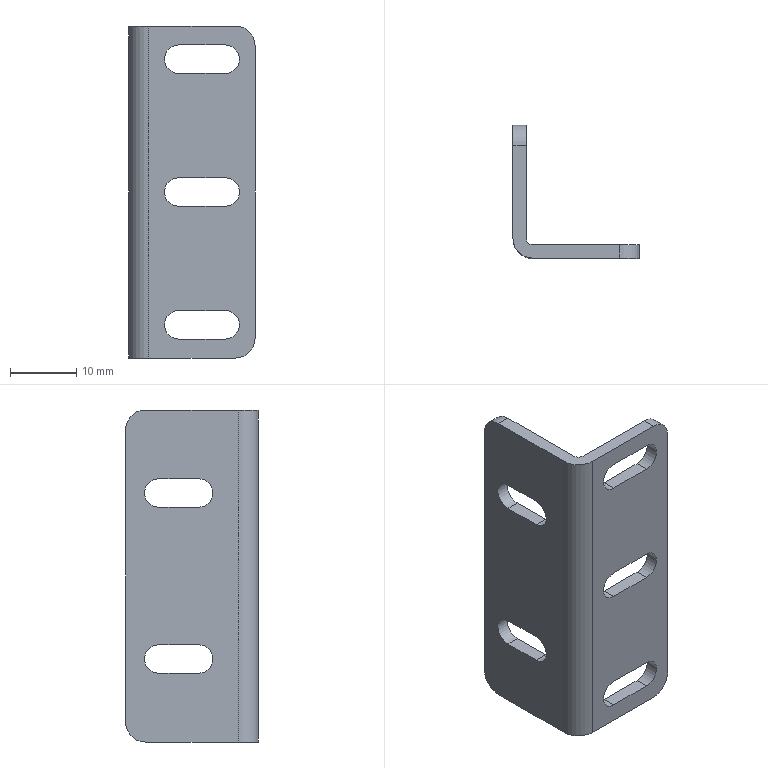Part | SolidWorks | features Fillet 3, ICE 2, ExtruThin 1 | 1 solid | 34 faces | box 19 x 20 x 50 mm | volume 3170 mm3 | plane 18 | cylinder 16 | commonest cylinder face diameters 4.3 x10 6 x5 2 x1
STEP:
#1=CARTESIAN_POINT('',(12.5,-2.,17.85));
#2=VERTEX_POINT('',#1);
#3=CARTESIAN_POINT('',(5.5,-2.,17.85));
#4=VERTEX_POINT('',#3);
#5=CARTESIAN_POINT('',(0.,-2.,17.85));
#6=DIRECTION('',(-1.,0.,0.));
#7=VECTOR('',#6,1000.);
#8=LINE('',#5,#7);
#9=EDGE_CURVE('',#2,#4,#8,.T.);
#10=ORIENTED_EDGE('',*,*,#9,.T.);
#11=CARTESIAN_POINT('',(5.5,-2.,22.15));
#12=VERTEX_POINT('',#11);
#13=CARTESIAN_POINT('',(5.5,-2.,20.));
#14=DIRECTION('',(0.,1.,0.));
#15=DIRECTION('',(0.,0.,1.));
#16=AXIS2_PLACEMENT_3D('',#13,#14,#15);
#17=CIRCLE('',#16,2.15);
#18=EDGE_CURVE('',#4,#12,#17,.T.);
#19=ORIENTED_EDGE('',*,*,#18,.T.);
#20=CARTESIAN_POINT('',(12.5,-2.,22.15));
#21=VERTEX_POINT('',#20);
#22=CARTESIAN_POINT('',(0.,-2.,22.15));
#23=DIRECTION('',(1.,0.,0.));
#24=VECTOR('',#23,1000.);
#25=LINE('',#22,#24);
#26=EDGE_CURVE('',#12,#21,#25,.T.);
#27=ORIENTED_EDGE('',*,*,#26,.T.);
#28=CARTESIAN_POINT('',(12.5,-2.,20.));
#29=DIRECTION('',(0.,1.,0.));
#30=DIRECTION('',(0.,0.,1.));
#31=AXIS2_PLACEMENT_3D('',#28,#29,#30);
#32=CIRCLE('',#31,2.15);
#33=EDGE_CURVE('',#21,#2,#32,.T.);
#34=ORIENTED_EDGE('',*,*,#33,.T.);
#35=EDGE_LOOP('',(#10,#19,#27,#34));
#36=FACE_BOUND('',#35,.T.);
#37=CARTESIAN_POINT('',(12.5,-2.,-2.15));
#38=VERTEX_POINT('',#37);
#39=CARTESIAN_POINT('',(5.5,-2.,-2.15));
#40=VERTEX_POINT('',#39);
#41=CARTESIAN_POINT('',(0.,-2.,-2.15));
#42=DIRECTION('',(-1.,0.,0.));
#43=VECTOR('',#42,1000.);
#44=LINE('',#41,#43);
#45=EDGE_CURVE('',#38,#40,#44,.T.);
#46=ORIENTED_EDGE('',*,*,#45,.T.);
#47=CARTESIAN_POINT('',(5.5,-2.,2.15));
#48=VERTEX_POINT('',#47);
#49=CARTESIAN_POINT('',(5.5,-2.,0.));
#50=DIRECTION('',(0.,1.,0.));
#51=DIRECTION('',(0.,0.,1.));
#52=AXIS2_PLACEMENT_3D('',#49,#50,#51);
#53=CIRCLE('',#52,2.15);
#54=EDGE_CURVE('',#40,#48,#53,.T.);
#55=ORIENTED_EDGE('',*,*,#54,.T.);
#56=CARTESIAN_POINT('',(12.5,-2.,2.15));
#57=VERTEX_POINT('',#56);
#58=CARTESIAN_POINT('',(0.,-2.,2.15));
#59=DIRECTION('',(1.,0.,0.));
#60=VECTOR('',#59,1000.);
#61=LINE('',#58,#60);
#62=EDGE_CURVE('',#48,#57,#61,.T.);
#63=ORIENTED_EDGE('',*,*,#62,.T.);
#64=CARTESIAN_POINT('',(12.5,-2.,0.));
#65=DIRECTION('',(0.,1.,0.));
#66=DIRECTION('',(0.,0.,1.));
#67=AXIS2_PLACEMENT_3D('',#64,#65,#66);
#68=CIRCLE('',#67,2.15);
#69=EDGE_CURVE('',#57,#38,#68,.T.);
#70=ORIENTED_EDGE('',*,*,#69,.T.);
#71=EDGE_LOOP('',(#46,#55,#63,#70));
#72=FACE_BOUND('',#71,.T.);
#73=CARTESIAN_POINT('',(12.5,-2.,-22.15));
#74=VERTEX_POINT('',#73);
#75=CARTESIAN_POINT('',(5.5,-2.,-22.15));
#76=VERTEX_POINT('',#75);
#77=CARTESIAN_POINT('',(0.,-2.,-22.15));
#78=DIRECTION('',(-1.,0.,0.));
#79=VECTOR('',#78,1000.);
#80=LINE('',#77,#79);
#81=EDGE_CURVE('',#74,#76,#80,.T.);
#82=ORIENTED_EDGE('',*,*,#81,.T.);
#83=CARTESIAN_POINT('',(5.5,-2.,-17.85));
#84=VERTEX_POINT('',#83);
#85=CARTESIAN_POINT('',(5.5,-2.,-20.));
#86=DIRECTION('',(0.,1.,0.));
#87=DIRECTION('',(0.,0.,1.));
#88=AXIS2_PLACEMENT_3D('',#85,#86,#87);
#89=CIRCLE('',#88,2.15);
#90=EDGE_CURVE('',#76,#84,#89,.T.);
#91=ORIENTED_EDGE('',*,*,#90,.T.);
#92=CARTESIAN_POINT('',(12.5,-2.,-17.85));
#93=VERTEX_POINT('',#92);
#94=CARTESIAN_POINT('',(0.,-2.,-17.85));
#95=DIRECTION('',(1.,0.,0.));
#96=VECTOR('',#95,1000.);
#97=LINE('',#94,#96);
#98=EDGE_CURVE('',#84,#93,#97,.T.);
#99=ORIENTED_EDGE('',*,*,#98,.T.);
#100=CARTESIAN_POINT('',(12.5,-2.,-20.));
#101=DIRECTION('',(0.,1.,0.));
#102=DIRECTION('',(0.,0.,1.));
#103=AXIS2_PLACEMENT_3D('',#100,#101,#102);
#104=CIRCLE('',#103,2.15);
#105=EDGE_CURVE('',#93,#74,#104,.T.);
#106=ORIENTED_EDGE('',*,*,#105,.T.);
#107=EDGE_LOOP('',(#82,#91,#99,#106));
#108=FACE_BOUND('',#107,.T.);
#109=CARTESIAN_POINT('',(1.,-2.,25.));
#110=VERTEX_POINT('',#109);
#111=CARTESIAN_POINT('',(14.,-2.,25.));
#112=VERTEX_POINT('',#111);
#113=CARTESIAN_POINT('',(0.,-2.,25.));
#114=DIRECTION('',(1.,0.,0.));
#115=VECTOR('',#114,1000.);
#116=LINE('',#113,#115);
#117=EDGE_CURVE('',#110,#112,#116,.T.);
#118=ORIENTED_EDGE('',*,*,#117,.F.);
#119=CARTESIAN_POINT('',(1.,-2.,-25.));
#120=VERTEX_POINT('',#119);
#121=CARTESIAN_POINT('',(1.,-2.,25.));
#122=DIRECTION('',(0.,0.,-1.));
#123=VECTOR('',#122,1000.);
#124=LINE('',#121,#123);
#125=EDGE_CURVE('',#110,#120,#124,.T.);
#126=ORIENTED_EDGE('',*,*,#125,.T.);
#127=CARTESIAN_POINT('',(14.,-2.,-25.));
#128=VERTEX_POINT('',#127);
#129=CARTESIAN_POINT('',(0.,-2.,-25.));
#130=DIRECTION('',(1.,0.,0.));
#131=VECTOR('',#130,1000.);
#132=LINE('',#129,#131);
#133=EDGE_CURVE('',#120,#128,#132,.T.);
#134=ORIENTED_EDGE('',*,*,#133,.T.);
#135=CARTESIAN_POINT('',(17.,-2.,-22.));
#136=VERTEX_POINT('',#135);
#137=CARTESIAN_POINT('',(14.,-2.,-22.));
#138=DIRECTION('',(0.,-1.,0.));
#139=DIRECTION('',(0.,0.,1.));
#140=AXIS2_PLACEMENT_3D('',#137,#138,#139);
#141=CIRCLE('',#140,3.);
#142=EDGE_CURVE('',#128,#136,#141,.T.);
#143=ORIENTED_EDGE('',*,*,#142,.T.);
#144=CARTESIAN_POINT('',(17.,-2.,22.));
#145=VERTEX_POINT('',#144);
#146=CARTESIAN_POINT('',(17.,-2.,25.));
#147=DIRECTION('',(0.,0.,-1.));
#148=VECTOR('',#147,1000.);
#149=LINE('',#146,#148);
#150=EDGE_CURVE('',#145,#136,#149,.T.);
#151=ORIENTED_EDGE('',*,*,#150,.F.);
#152=CARTESIAN_POINT('',(14.,-2.,22.));
#153=DIRECTION('',(0.,-1.,0.));
#154=DIRECTION('',(0.,0.,1.));
#155=AXIS2_PLACEMENT_3D('',#152,#153,#154);
#156=CIRCLE('',#155,3.);
#157=EDGE_CURVE('',#145,#112,#156,.T.);
#158=ORIENTED_EDGE('',*,*,#157,.T.);
#159=EDGE_LOOP('',(#118,#126,#134,#143,#151,#158));
#160=FACE_OUTER_BOUND('',#159,.T.);
#161=CARTESIAN_POINT('',(0.,-2.,25.));
#162=DIRECTION('',(0.,1.,0.));
#163=DIRECTION('',(0.,0.,1.));
#164=AXIS2_PLACEMENT_3D('',#161,#162,#163);
#165=PLANE('',#164);
#166=ADVANCED_FACE('',(#36,#72,#108,#160),#165,.F.);
#167=CARTESIAN_POINT('',(17.,0.,22.));
#168=VERTEX_POINT('',#167);
#169=CARTESIAN_POINT('',(17.,0.,-22.));
#170=VERTEX_POINT('',#169);
#171=CARTESIAN_POINT('',(17.,0.,25.));
#172=DIRECTION('',(0.,0.,-1.));
#173=VECTOR('',#172,1000.);
#174=LINE('',#171,#173);
#175=EDGE_CURVE('',#168,#170,#174,.T.);
#176=ORIENTED_EDGE('',*,*,#175,.F.);
#177=CARTESIAN_POINT('',(17.,-2.,22.));
#178=DIRECTION('',(0.,-1.,0.));
#179=VECTOR('',#178,1000.);
#180=LINE('',#177,#179);
#181=EDGE_CURVE('',#168,#145,#180,.T.);
#182=ORIENTED_EDGE('',*,*,#181,.T.);
#183=ORIENTED_EDGE('',*,*,#150,.T.);
#184=CARTESIAN_POINT('',(17.,0.,-22.));
#185=DIRECTION('',(0.,1.,0.));
#186=VECTOR('',#185,1000.);
#187=LINE('',#184,#186);
#188=EDGE_CURVE('',#136,#170,#187,.T.);
#189=ORIENTED_EDGE('',*,*,#188,.T.);
#190=EDGE_LOOP('',(#176,#182,#183,#189));
#191=FACE_OUTER_BOUND('',#190,.T.);
#192=CARTESIAN_POINT('',(17.,0.,25.));
#193=DIRECTION('',(1.,0.,0.));
#194=DIRECTION('',(0.,0.,-1.));
#195=AXIS2_PLACEMENT_3D('',#192,#193,#194);
#196=PLANE('',#195);
#197=ADVANCED_FACE('',(#191),#196,.T.);
#198=CARTESIAN_POINT('',(5.5,0.,17.85));
#199=VERTEX_POINT('',#198);
#200=CARTESIAN_POINT('',(5.5,0.,22.15));
#201=VERTEX_POINT('',#200);
#202=CARTESIAN_POINT('',(5.5,0.,20.));
#203=DIRECTION('',(0.,1.,0.));
#204=DIRECTION('',(0.,0.,-1.));
#205=AXIS2_PLACEMENT_3D('',#202,#203,#204);
#206=CIRCLE('',#205,2.15);
#207=EDGE_CURVE('',#199,#201,#206,.T.);
#208=ORIENTED_EDGE('',*,*,#207,.F.);
#209=CARTESIAN_POINT('',(12.5,0.,17.85));
#210=VERTEX_POINT('',#209);
#211=CARTESIAN_POINT('',(5.5,0.,17.85));
#212=DIRECTION('',(-1.,0.,0.));
#213=VECTOR('',#212,1000.);
#214=LINE('',#211,#213);
#215=EDGE_CURVE('',#210,#199,#214,.T.);
#216=ORIENTED_EDGE('',*,*,#215,.F.);
#217=CARTESIAN_POINT('',(12.5,0.,22.15));
#218=VERTEX_POINT('',#217);
#219=CARTESIAN_POINT('',(12.5,0.,20.));
#220=DIRECTION('',(0.,1.,0.));
#221=DIRECTION('',(0.,0.,-1.));
#222=AXIS2_PLACEMENT_3D('',#219,#220,#221);
#223=CIRCLE('',#222,2.15);
#224=EDGE_CURVE('',#218,#210,#223,.T.);
#225=ORIENTED_EDGE('',*,*,#224,.F.);
#226=CARTESIAN_POINT('',(5.5,0.,22.15));
#227=DIRECTION('',(1.,0.,0.));
#228=VECTOR('',#227,1000.);
#229=LINE('',#226,#228);
#230=EDGE_CURVE('',#201,#218,#229,.T.);
#231=ORIENTED_EDGE('',*,*,#230,.F.);
#232=EDGE_LOOP('',(#208,#216,#225,#231));
#233=FACE_BOUND('',#232,.T.);
#234=CARTESIAN_POINT('',(5.5,0.,-2.15));
#235=VERTEX_POINT('',#234);
#236=CARTESIAN_POINT('',(5.5,0.,2.15));
#237=VERTEX_POINT('',#236);
#238=CARTESIAN_POINT('',(5.5,0.,0.));
#239=DIRECTION('',(0.,1.,0.));
#240=DIRECTION('',(0.,0.,1.));
#241=AXIS2_PLACEMENT_3D('',#238,#239,#240);
#242=CIRCLE('',#241,2.15);
#243=EDGE_CURVE('',#235,#237,#242,.T.);
#244=ORIENTED_EDGE('',*,*,#243,.F.);
#245=CARTESIAN_POINT('',(12.5,0.,-2.15));
#246=VERTEX_POINT('',#245);
#247=CARTESIAN_POINT('',(5.5,0.,-2.15));
#248=DIRECTION('',(-1.,0.,0.));
#249=VECTOR('',#248,1000.);
#250=LINE('',#247,#249);
#251=EDGE_CURVE('',#246,#235,#250,.T.);
#252=ORIENTED_EDGE('',*,*,#251,.F.);
#253=CARTESIAN_POINT('',(12.5,0.,2.15));
#254=VERTEX_POINT('',#253);
#255=CARTESIAN_POINT('',(12.5,0.,0.));
#256=DIRECTION('',(0.,1.,0.));
#257=DIRECTION('',(0.,0.,1.));
#258=AXIS2_PLACEMENT_3D('',#255,#256,#257);
#259=CIRCLE('',#258,2.15);
#260=EDGE_CURVE('',#254,#246,#259,.T.);
#261=ORIENTED_EDGE('',*,*,#260,.F.);
#262=CARTESIAN_POINT('',(5.5,0.,2.15));
#263=DIRECTION('',(1.,0.,0.));
#264=VECTOR('',#263,1000.);
#265=LINE('',#262,#264);
#266=EDGE_CURVE('',#237,#254,#265,.T.);
#267=ORIENTED_EDGE('',*,*,#266,.F.);
#268=EDGE_LOOP('',(#244,#252,#261,#267));
#269=FACE_BOUND('',#268,.T.);
#270=CARTESIAN_POINT('',(5.5,0.,-22.15));
#271=VERTEX_POINT('',#270);
#272=CARTESIAN_POINT('',(5.5,0.,-17.85));
#273=VERTEX_POINT('',#272);
#274=CARTESIAN_POINT('',(5.5,0.,-20.));
#275=DIRECTION('',(0.,1.,0.));
#276=DIRECTION('',(0.,0.,1.));
#277=AXIS2_PLACEMENT_3D('',#274,#275,#276);
#278=CIRCLE('',#277,2.15);
#279=EDGE_CURVE('',#271,#273,#278,.T.);
#280=ORIENTED_EDGE('',*,*,#279,.F.);
#281=CARTESIAN_POINT('',(12.5,0.,-22.15));
#282=VERTEX_POINT('',#281);
#283=CARTESIAN_POINT('',(5.5,0.,-22.15));
#284=DIRECTION('',(-1.,0.,0.));
#285=VECTOR('',#284,1000.);
#286=LINE('',#283,#285);
#287=EDGE_CURVE('',#282,#271,#286,.T.);
#288=ORIENTED_EDGE('',*,*,#287,.F.);
#289=CARTESIAN_POINT('',(12.5,0.,-17.85));
#290=VERTEX_POINT('',#289);
#291=CARTESIAN_POINT('',(12.5,0.,-20.));
#292=DIRECTION('',(0.,1.,0.));
#293=DIRECTION('',(0.,0.,1.));
#294=AXIS2_PLACEMENT_3D('',#291,#292,#293);
#295=CIRCLE('',#294,2.15);
#296=EDGE_CURVE('',#290,#282,#295,.T.);
#297=ORIENTED_EDGE('',*,*,#296,.F.);
#298=CARTESIAN_POINT('',(5.5,0.,-17.85));
#299=DIRECTION('',(1.,0.,0.));
#300=VECTOR('',#299,1000.);
#301=LINE('',#298,#300);
#302=EDGE_CURVE('',#273,#290,#301,.T.);
#303=ORIENTED_EDGE('',*,*,#302,.F.);
#304=EDGE_LOOP('',(#280,#288,#297,#303));
#305=FACE_BOUND('',#304,.T.);
#306=CARTESIAN_POINT('',(1.,0.,-25.));
#307=VERTEX_POINT('',#306);
#308=CARTESIAN_POINT('',(14.,0.,-25.));
#309=VERTEX_POINT('',#308);
#310=CARTESIAN_POINT('',(0.,0.,-25.));
#311=DIRECTION('',(1.,0.,0.));
#312=VECTOR('',#311,1000.);
#313=LINE('',#310,#312);
#314=EDGE_CURVE('',#307,#309,#313,.T.);
#315=ORIENTED_EDGE('',*,*,#314,.F.);
#316=CARTESIAN_POINT('',(1.,0.,25.));
#317=VERTEX_POINT('',#316);
#318=CARTESIAN_POINT('',(1.,0.,25.));
#319=DIRECTION('',(0.,0.,1.));
#320=VECTOR('',#319,1000.);
#321=LINE('',#318,#320);
#322=EDGE_CURVE('',#307,#317,#321,.T.);
#323=ORIENTED_EDGE('',*,*,#322,.T.);
#324=CARTESIAN_POINT('',(14.,0.,25.));
#325=VERTEX_POINT('',#324);
#326=CARTESIAN_POINT('',(0.,0.,25.));
#327=DIRECTION('',(1.,0.,0.));
#328=VECTOR('',#327,1000.);
#329=LINE('',#326,#328);
#330=EDGE_CURVE('',#317,#325,#329,.T.);
#331=ORIENTED_EDGE('',*,*,#330,.T.);
#332=CARTESIAN_POINT('',(14.,0.,22.));
#333=DIRECTION('',(0.,1.,0.));
#334=DIRECTION('',(0.,0.,1.));
#335=AXIS2_PLACEMENT_3D('',#332,#333,#334);
#336=CIRCLE('',#335,3.);
#337=EDGE_CURVE('',#325,#168,#336,.T.);
#338=ORIENTED_EDGE('',*,*,#337,.T.);
#339=ORIENTED_EDGE('',*,*,#175,.T.);
#340=CARTESIAN_POINT('',(14.,0.,-22.));
#341=DIRECTION('',(0.,1.,0.));
#342=DIRECTION('',(0.,0.,1.));
#343=AXIS2_PLACEMENT_3D('',#340,#341,#342);
#344=CIRCLE('',#343,3.);
#345=EDGE_CURVE('',#170,#309,#344,.T.);
#346=ORIENTED_EDGE('',*,*,#345,.T.);
#347=EDGE_LOOP('',(#315,#323,#331,#338,#339,#346));
#348=FACE_OUTER_BOUND('',#347,.T.);
#349=CARTESIAN_POINT('',(0.,0.,25.));
#350=DIRECTION('',(0.,1.,0.));
#351=DIRECTION('',(0.,0.,1.));
#352=AXIS2_PLACEMENT_3D('',#349,#350,#351);
#353=PLANE('',#352);
#354=ADVANCED_FACE('',(#233,#269,#305,#348),#353,.T.);
#355=CARTESIAN_POINT('',(0.,13.,-14.65));
#356=VERTEX_POINT('',#355);
#357=CARTESIAN_POINT('',(0.,13.,-10.35));
#358=VERTEX_POINT('',#357);
#359=CARTESIAN_POINT('',(0.,13.,-12.5));
#360=DIRECTION('',(1.,0.,0.));
#361=DIRECTION('',(0.,0.,1.));
#362=AXIS2_PLACEMENT_3D('',#359,#360,#361);
#363=CIRCLE('',#362,2.15);
#364=EDGE_CURVE('',#356,#358,#363,.T.);
#365=ORIENTED_EDGE('',*,*,#364,.F.);
#366=CARTESIAN_POINT('',(0.,7.,-14.65));
#367=VERTEX_POINT('',#366);
#368=CARTESIAN_POINT('',(0.,13.,-14.65));
#369=DIRECTION('',(0.,1.,0.));
#370=VECTOR('',#369,1000.);
#371=LINE('',#368,#370);
#372=EDGE_CURVE('',#367,#356,#371,.T.);
#373=ORIENTED_EDGE('',*,*,#372,.F.);
#374=CARTESIAN_POINT('',(0.,7.,-10.35));
#375=VERTEX_POINT('',#374);
#376=CARTESIAN_POINT('',(0.,7.,-12.5));
#377=DIRECTION('',(1.,0.,0.));
#378=DIRECTION('',(0.,0.,1.));
#379=AXIS2_PLACEMENT_3D('',#376,#377,#378);
#380=CIRCLE('',#379,2.15);
#381=EDGE_CURVE('',#375,#367,#380,.T.);
#382=ORIENTED_EDGE('',*,*,#381,.F.);
#383=CARTESIAN_POINT('',(0.,13.,-10.35));
#384=DIRECTION('',(0.,-1.,0.));
#385=VECTOR('',#384,1000.);
#386=LINE('',#383,#385);
#387=EDGE_CURVE('',#358,#375,#386,.T.);
#388=ORIENTED_EDGE('',*,*,#387,.F.);
#389=EDGE_LOOP('',(#365,#373,#382,#388));
#390=FACE_BOUND('',#389,.T.);
#391=CARTESIAN_POINT('',(0.,13.,10.35));
#392=VERTEX_POINT('',#391);
#393=CARTESIAN_POINT('',(0.,13.,14.65));
#394=VERTEX_POINT('',#393);
#395=CARTESIAN_POINT('',(0.,13.,12.5));
#396=DIRECTION('',(1.,0.,0.));
#397=DIRECTION('',(0.,0.,-1.));
#398=AXIS2_PLACEMENT_3D('',#395,#396,#397);
#399=CIRCLE('',#398,2.15);
#400=EDGE_CURVE('',#392,#394,#399,.T.);
#401=ORIENTED_EDGE('',*,*,#400,.F.);
#402=CARTESIAN_POINT('',(0.,7.,10.35));
#403=VERTEX_POINT('',#402);
#404=CARTESIAN_POINT('',(0.,13.,10.35));
#405=DIRECTION('',(0.,1.,0.));
#406=VECTOR('',#405,1000.);
#407=LINE('',#404,#406);
#408=EDGE_CURVE('',#403,#392,#407,.T.);
#409=ORIENTED_EDGE('',*,*,#408,.F.);
#410=CARTESIAN_POINT('',(0.,7.,14.65));
#411=VERTEX_POINT('',#410);
#412=CARTESIAN_POINT('',(0.,7.,12.5));
#413=DIRECTION('',(1.,0.,0.));
#414=DIRECTION('',(0.,0.,-1.));
#415=AXIS2_PLACEMENT_3D('',#412,#413,#414);
#416=CIRCLE('',#415,2.15);
#417=EDGE_CURVE('',#411,#403,#416,.T.);
#418=ORIENTED_EDGE('',*,*,#417,.F.);
#419=CARTESIAN_POINT('',(0.,13.,14.65));
#420=DIRECTION('',(0.,-1.,0.));
#421=VECTOR('',#420,1000.);
#422=LINE('',#419,#421);
#423=EDGE_CURVE('',#394,#411,#422,.T.);
#424=ORIENTED_EDGE('',*,*,#423,.F.);
#425=EDGE_LOOP('',(#401,#409,#418,#424));
#426=FACE_BOUND('',#425,.T.);
#427=CARTESIAN_POINT('',(0.,15.,25.));
#428=VERTEX_POINT('',#427);
#429=CARTESIAN_POINT('',(0.,1.,25.));
#430=VERTEX_POINT('',#429);
#431=CARTESIAN_POINT('',(0.,0.,25.));
#432=DIRECTION('',(0.,-1.,0.));
#433=VECTOR('',#432,1000.);
#434=LINE('',#431,#433);
#435=EDGE_CURVE('',#428,#430,#434,.T.);
#436=ORIENTED_EDGE('',*,*,#435,.T.);
#437=CARTESIAN_POINT('',(0.,1.,-25.));
#438=VERTEX_POINT('',#437);
#439=CARTESIAN_POINT('',(0.,1.,-25.));
#440=DIRECTION('',(0.,0.,-1.));
#441=VECTOR('',#440,1000.);
#442=LINE('',#439,#441);
#443=EDGE_CURVE('',#430,#438,#442,.T.);
#444=ORIENTED_EDGE('',*,*,#443,.T.);
#445=CARTESIAN_POINT('',(0.,15.,-25.));
#446=VERTEX_POINT('',#445);
#447=CARTESIAN_POINT('',(0.,0.,-25.));
#448=DIRECTION('',(0.,-1.,0.));
#449=VECTOR('',#448,1000.);
#450=LINE('',#447,#449);
#451=EDGE_CURVE('',#446,#438,#450,.T.);
#452=ORIENTED_EDGE('',*,*,#451,.F.);
#453=CARTESIAN_POINT('',(0.,18.,-22.));
#454=VERTEX_POINT('',#453);
#455=CARTESIAN_POINT('',(0.,15.,-22.));
#456=DIRECTION('',(1.,0.,0.));
#457=DIRECTION('',(0.,0.,-1.));
#458=AXIS2_PLACEMENT_3D('',#455,#456,#457);
#459=CIRCLE('',#458,3.);
#460=EDGE_CURVE('',#446,#454,#459,.T.);
#461=ORIENTED_EDGE('',*,*,#460,.T.);
#462=CARTESIAN_POINT('',(0.,18.,22.));
#463=VERTEX_POINT('',#462);
#464=CARTESIAN_POINT('',(0.,18.,25.));
#465=DIRECTION('',(0.,0.,-1.));
#466=VECTOR('',#465,1000.);
#467=LINE('',#464,#466);
#468=EDGE_CURVE('',#463,#454,#467,.T.);
#469=ORIENTED_EDGE('',*,*,#468,.F.);
#470=CARTESIAN_POINT('',(0.,15.,22.));
#471=DIRECTION('',(1.,0.,0.));
#472=DIRECTION('',(0.,0.,-1.));
#473=AXIS2_PLACEMENT_3D('',#470,#471,#472);
#474=CIRCLE('',#473,3.);
#475=EDGE_CURVE('',#463,#428,#474,.T.);
#476=ORIENTED_EDGE('',*,*,#475,.T.);
#477=EDGE_LOOP('',(#436,#444,#452,#461,#469,#476));
#478=FACE_OUTER_BOUND('',#477,.T.);
#479=CARTESIAN_POINT('',(0.,0.,25.));
#480=DIRECTION('',(1.,0.,0.));
#481=DIRECTION('',(0.,0.,-1.));
#482=AXIS2_PLACEMENT_3D('',#479,#480,#481);
#483=PLANE('',#482);
#484=ADVANCED_FACE('',(#390,#426,#478),#483,.T.);
#485=CARTESIAN_POINT('',(-2.,18.,22.));
#486=VERTEX_POINT('',#485);
#487=CARTESIAN_POINT('',(-2.,18.,-22.));
#488=VERTEX_POINT('',#487);
#489=CARTESIAN_POINT('',(-2.,18.,25.));
#490=DIRECTION('',(0.,0.,-1.));
#491=VECTOR('',#490,1000.);
#492=LINE('',#489,#491);
#493=EDGE_CURVE('',#486,#488,#492,.T.);
#494=ORIENTED_EDGE('',*,*,#493,.F.);
#495=CARTESIAN_POINT('',(0.,18.,22.));
#496=DIRECTION('',(1.,0.,0.));
#497=VECTOR('',#496,1000.);
#498=LINE('',#495,#497);
#499=EDGE_CURVE('',#486,#463,#498,.T.);
#500=ORIENTED_EDGE('',*,*,#499,.T.);
#501=ORIENTED_EDGE('',*,*,#468,.T.);
#502=CARTESIAN_POINT('',(-2.,18.,-22.));
#503=DIRECTION('',(-1.,0.,0.));
#504=VECTOR('',#503,1000.);
#505=LINE('',#502,#504);
#506=EDGE_CURVE('',#454,#488,#505,.T.);
#507=ORIENTED_EDGE('',*,*,#506,.T.);
#508=EDGE_LOOP('',(#494,#500,#501,#507));
#509=FACE_OUTER_BOUND('',#508,.T.);
#510=CARTESIAN_POINT('',(-2.,18.,25.));
#511=DIRECTION('',(0.,1.,0.));
#512=DIRECTION('',(0.,0.,1.));
#513=AXIS2_PLACEMENT_3D('',#510,#511,#512);
#514=PLANE('',#513);
#515=ADVANCED_FACE('',(#509),#514,.T.);
#516=CARTESIAN_POINT('',(-2.,7.,-14.65));
#517=VERTEX_POINT('',#516);
#518=CARTESIAN_POINT('',(-2.,13.,-14.65));
#519=VERTEX_POINT('',#518);
#520=CARTESIAN_POINT('',(-2.,0.,-14.65));
#521=DIRECTION('',(0.,1.,0.));
#522=VECTOR('',#521,1000.);
#523=LINE('',#520,#522);
#524=EDGE_CURVE('',#517,#519,#523,.T.);
#525=ORIENTED_EDGE('',*,*,#524,.T.);
#526=CARTESIAN_POINT('',(-2.,13.,-10.35));
#527=VERTEX_POINT('',#526);
#528=CARTESIAN_POINT('',(-2.,13.,-12.5));
#529=DIRECTION('',(1.,0.,0.));
#530=DIRECTION('',(0.,0.,-1.));
#531=AXIS2_PLACEMENT_3D('',#528,#529,#530);
#532=CIRCLE('',#531,2.15);
#533=EDGE_CURVE('',#519,#527,#532,.T.);
#534=ORIENTED_EDGE('',*,*,#533,.T.);
#535=CARTESIAN_POINT('',(-2.,7.,-10.35));
#536=VERTEX_POINT('',#535);
#537=CARTESIAN_POINT('',(-2.,0.,-10.35));
#538=DIRECTION('',(0.,-1.,0.));
#539=VECTOR('',#538,1000.);
#540=LINE('',#537,#539);
#541=EDGE_CURVE('',#527,#536,#540,.T.);
#542=ORIENTED_EDGE('',*,*,#541,.T.);
#543=CARTESIAN_POINT('',(-2.,7.,-12.5));
#544=DIRECTION('',(1.,0.,0.));
#545=DIRECTION('',(0.,0.,-1.));
#546=AXIS2_PLACEMENT_3D('',#543,#544,#545);
#547=CIRCLE('',#546,2.15);
#548=EDGE_CURVE('',#536,#517,#547,.T.);
#549=ORIENTED_EDGE('',*,*,#548,.T.);
#550=EDGE_LOOP('',(#525,#534,#542,#549));
#551=FACE_BOUND('',#550,.T.);
#552=CARTESIAN_POINT('',(-2.,7.,10.35));
#553=VERTEX_POINT('',#552);
#554=CARTESIAN_POINT('',(-2.,13.,10.35));
#555=VERTEX_POINT('',#554);
#556=CARTESIAN_POINT('',(-2.,0.,10.35));
#557=DIRECTION('',(0.,1.,0.));
#558=VECTOR('',#557,1000.);
#559=LINE('',#556,#558);
#560=EDGE_CURVE('',#553,#555,#559,.T.);
#561=ORIENTED_EDGE('',*,*,#560,.T.);
#562=CARTESIAN_POINT('',(-2.,13.,14.65));
#563=VERTEX_POINT('',#562);
#564=CARTESIAN_POINT('',(-2.,13.,12.5));
#565=DIRECTION('',(1.,0.,0.));
#566=DIRECTION('',(0.,0.,-1.));
#567=AXIS2_PLACEMENT_3D('',#564,#565,#566);
#568=CIRCLE('',#567,2.15);
#569=EDGE_CURVE('',#555,#563,#568,.T.);
#570=ORIENTED_EDGE('',*,*,#569,.T.);
#571=CARTESIAN_POINT('',(-2.,7.,14.65));
#572=VERTEX_POINT('',#571);
#573=CARTESIAN_POINT('',(-2.,0.,14.65));
#574=DIRECTION('',(0.,-1.,0.));
#575=VECTOR('',#574,1000.);
#576=LINE('',#573,#575);
#577=EDGE_CURVE('',#563,#572,#576,.T.);
#578=ORIENTED_EDGE('',*,*,#577,.T.);
#579=CARTESIAN_POINT('',(-2.,7.,12.5));
#580=DIRECTION('',(1.,0.,0.));
#581=DIRECTION('',(0.,0.,-1.));
#582=AXIS2_PLACEMENT_3D('',#579,#580,#581);
#583=CIRCLE('',#582,2.15);
#584=EDGE_CURVE('',#572,#553,#583,.T.);
#585=ORIENTED_EDGE('',*,*,#584,.T.);
#586=EDGE_LOOP('',(#561,#570,#578,#585));
#587=FACE_BOUND('',#586,.T.);
#588=CARTESIAN_POINT('',(-2.,15.,-25.));
#589=VERTEX_POINT('',#588);
#590=CARTESIAN_POINT('',(-2.,1.,-25.));
#591=VERTEX_POINT('',#590);
#592=CARTESIAN_POINT('',(-2.,0.,-25.));
#593=DIRECTION('',(0.,-1.,0.));
#594=VECTOR('',#593,1000.);
#595=LINE('',#592,#594);
#596=EDGE_CURVE('',#589,#591,#595,.T.);
#597=ORIENTED_EDGE('',*,*,#596,.T.);
#598=CARTESIAN_POINT('',(-2.,1.,25.));
#599=VERTEX_POINT('',#598);
#600=CARTESIAN_POINT('',(-2.,1.,25.));
#601=DIRECTION('',(0.,0.,1.));
#602=VECTOR('',#601,1000.);
#603=LINE('',#600,#602);
#604=EDGE_CURVE('',#591,#599,#603,.T.);
#605=ORIENTED_EDGE('',*,*,#604,.T.);
#606=CARTESIAN_POINT('',(-2.,15.,25.));
#607=VERTEX_POINT('',#606);
#608=CARTESIAN_POINT('',(-2.,0.,25.));
#609=DIRECTION('',(0.,-1.,0.));
#610=VECTOR('',#609,1000.);
#611=LINE('',#608,#610);
#612=EDGE_CURVE('',#607,#599,#611,.T.);
#613=ORIENTED_EDGE('',*,*,#612,.F.);
#614=CARTESIAN_POINT('',(-2.,15.,22.));
#615=DIRECTION('',(-1.,0.,0.));
#616=DIRECTION('',(0.,0.,-1.));
#617=AXIS2_PLACEMENT_3D('',#614,#615,#616);
#618=CIRCLE('',#617,3.);
#619=EDGE_CURVE('',#607,#486,#618,.T.);
#620=ORIENTED_EDGE('',*,*,#619,.T.);
#621=ORIENTED_EDGE('',*,*,#493,.T.);
#622=CARTESIAN_POINT('',(-2.,15.,-22.));
#623=DIRECTION('',(-1.,0.,0.));
#624=DIRECTION('',(0.,0.,-1.));
#625=AXIS2_PLACEMENT_3D('',#622,#623,#624);
#626=CIRCLE('',#625,3.);
#627=EDGE_CURVE('',#488,#589,#626,.T.);
#628=ORIENTED_EDGE('',*,*,#627,.T.);
#629=EDGE_LOOP('',(#597,#605,#613,#620,#621,#628));
#630=FACE_OUTER_BOUND('',#629,.T.);
#631=CARTESIAN_POINT('',(-2.,0.,25.));
#632=DIRECTION('',(1.,0.,0.));
#633=DIRECTION('',(0.,0.,-1.));
#634=AXIS2_PLACEMENT_3D('',#631,#632,#633);
#635=PLANE('',#634);
#636=ADVANCED_FACE('',(#551,#587,#630),#635,.F.);
#637=ORIENTED_EDGE('',*,*,#612,.T.);
#638=CARTESIAN_POINT('',(1.,1.,25.));
#639=DIRECTION('',(0.,0.,1.));
#640=DIRECTION('',(-1.,0.,0.));
#641=AXIS2_PLACEMENT_3D('',#638,#639,#640);
#642=CIRCLE('',#641,3.);
#643=EDGE_CURVE('',#599,#110,#642,.T.);
#644=ORIENTED_EDGE('',*,*,#643,.T.);
#645=ORIENTED_EDGE('',*,*,#117,.T.);
#646=CARTESIAN_POINT('',(14.,0.,25.));
#647=DIRECTION('',(0.,1.,0.));
#648=VECTOR('',#647,1000.);
#649=LINE('',#646,#648);
#650=EDGE_CURVE('',#112,#325,#649,.T.);
#651=ORIENTED_EDGE('',*,*,#650,.T.);
#652=ORIENTED_EDGE('',*,*,#330,.F.);
#653=CARTESIAN_POINT('',(1.,1.,25.));
#654=DIRECTION('',(0.,0.,-1.));
#655=DIRECTION('',(-1.,0.,0.));
#656=AXIS2_PLACEMENT_3D('',#653,#654,#655);
#657=CIRCLE('',#656,1.);
#658=EDGE_CURVE('',#317,#430,#657,.T.);
#659=ORIENTED_EDGE('',*,*,#658,.T.);
#660=ORIENTED_EDGE('',*,*,#435,.F.);
#661=CARTESIAN_POINT('',(-2.,15.,25.));
#662=DIRECTION('',(-1.,0.,0.));
#663=VECTOR('',#662,1000.);
#664=LINE('',#661,#663);
#665=EDGE_CURVE('',#428,#607,#664,.T.);
#666=ORIENTED_EDGE('',*,*,#665,.T.);
#667=EDGE_LOOP('',(#637,#644,#645,#651,#652,#659,#660,#666));
#668=FACE_OUTER_BOUND('',#667,.T.);
#669=CARTESIAN_POINT('',(0.,0.,25.));
#670=DIRECTION('',(0.,0.,-1.));
#671=DIRECTION('',(-1.,0.,0.));
#672=AXIS2_PLACEMENT_3D('',#669,#670,#671);
#673=PLANE('',#672);
#674=ADVANCED_FACE('',(#668),#673,.F.);
#675=ORIENTED_EDGE('',*,*,#133,.F.);
#676=CARTESIAN_POINT('',(1.,1.,-25.));
#677=DIRECTION('',(0.,0.,-1.));
#678=DIRECTION('',(-1.,0.,0.));
#679=AXIS2_PLACEMENT_3D('',#676,#677,#678);
#680=CIRCLE('',#679,3.);
#681=EDGE_CURVE('',#120,#591,#680,.T.);
#682=ORIENTED_EDGE('',*,*,#681,.T.);
#683=ORIENTED_EDGE('',*,*,#596,.F.);
#684=CARTESIAN_POINT('',(0.,15.,-25.));
#685=DIRECTION('',(1.,0.,0.));
#686=VECTOR('',#685,1000.);
#687=LINE('',#684,#686);
#688=EDGE_CURVE('',#589,#446,#687,.T.);
#689=ORIENTED_EDGE('',*,*,#688,.T.);
#690=ORIENTED_EDGE('',*,*,#451,.T.);
#691=CARTESIAN_POINT('',(1.,1.,-25.));
#692=DIRECTION('',(0.,0.,1.));
#693=DIRECTION('',(-1.,0.,0.));
#694=AXIS2_PLACEMENT_3D('',#691,#692,#693);
#695=CIRCLE('',#694,1.);
#696=EDGE_CURVE('',#438,#307,#695,.T.);
#697=ORIENTED_EDGE('',*,*,#696,.T.);
#698=ORIENTED_EDGE('',*,*,#314,.T.);
#699=CARTESIAN_POINT('',(14.,0.,-25.));
#700=DIRECTION('',(0.,-1.,0.));
#701=VECTOR('',#700,1000.);
#702=LINE('',#699,#701);
#703=EDGE_CURVE('',#309,#128,#702,.T.);
#704=ORIENTED_EDGE('',*,*,#703,.T.);
#705=EDGE_LOOP('',(#675,#682,#683,#689,#690,#697,#698,#704));
#706=FACE_OUTER_BOUND('',#705,.T.);
#707=CARTESIAN_POINT('',(0.,0.,-25.));
#708=DIRECTION('',(0.,0.,-1.));
#709=DIRECTION('',(-1.,0.,0.));
#710=AXIS2_PLACEMENT_3D('',#707,#708,#709);
#711=PLANE('',#710);
#712=ADVANCED_FACE('',(#706),#711,.T.);
#713=CARTESIAN_POINT('',(5.5,-10.,-22.15));
#714=DIRECTION('',(0.,1.,0.));
#715=VECTOR('',#714,1000.);
#716=LINE('',#713,#715);
#717=EDGE_CURVE('',#76,#271,#716,.T.);
#718=ORIENTED_EDGE('',*,*,#717,.T.);
#719=ORIENTED_EDGE('',*,*,#279,.T.);
#720=CARTESIAN_POINT('',(5.5,-10.,-17.85));
#721=DIRECTION('',(0.,1.,0.));
#722=VECTOR('',#721,1000.);
#723=LINE('',#720,#722);
#724=EDGE_CURVE('',#84,#273,#723,.T.);
#725=ORIENTED_EDGE('',*,*,#724,.F.);
#726=ORIENTED_EDGE('',*,*,#90,.F.);
#727=EDGE_LOOP('',(#718,#719,#725,#726));
#728=FACE_OUTER_BOUND('',#727,.T.);
#729=CARTESIAN_POINT('',(5.5,-10.,-20.));
#730=DIRECTION('',(0.,1.,0.));
#731=DIRECTION('',(0.,0.,1.));
#732=AXIS2_PLACEMENT_3D('',#729,#730,#731);
#733=CYLINDRICAL_SURFACE('',#732,2.15);
#734=ADVANCED_FACE('',(#728),#733,.F.);
#735=CARTESIAN_POINT('',(12.5,-10.,-22.15));
#736=DIRECTION('',(0.,1.,0.));
#737=VECTOR('',#736,1000.);
#738=LINE('',#735,#737);
#739=EDGE_CURVE('',#74,#282,#738,.T.);
#740=ORIENTED_EDGE('',*,*,#739,.T.);
#741=ORIENTED_EDGE('',*,*,#287,.T.);
#742=ORIENTED_EDGE('',*,*,#717,.F.);
#743=ORIENTED_EDGE('',*,*,#81,.F.);
#744=EDGE_LOOP('',(#740,#741,#742,#743));
#745=FACE_OUTER_BOUND('',#744,.T.);
#746=CARTESIAN_POINT('',(5.5,-10.,-22.15));
#747=DIRECTION('',(0.,0.,-1.));
#748=DIRECTION('',(-1.,0.,0.));
#749=AXIS2_PLACEMENT_3D('',#746,#747,#748);
#750=PLANE('',#749);
#751=ADVANCED_FACE('',(#745),#750,.F.);
#752=CARTESIAN_POINT('',(12.5,-10.,-17.85));
#753=DIRECTION('',(0.,1.,0.));
#754=VECTOR('',#753,1000.);
#755=LINE('',#752,#754);
#756=EDGE_CURVE('',#93,#290,#755,.T.);
#757=ORIENTED_EDGE('',*,*,#756,.T.);
#758=ORIENTED_EDGE('',*,*,#296,.T.);
#759=ORIENTED_EDGE('',*,*,#739,.F.);
#760=ORIENTED_EDGE('',*,*,#105,.F.);
#761=EDGE_LOOP('',(#757,#758,#759,#760));
#762=FACE_OUTER_BOUND('',#761,.T.);
#763=CARTESIAN_POINT('',(12.5,-10.,-20.));
#764=DIRECTION('',(0.,1.,0.));
#765=DIRECTION('',(0.,0.,1.));
#766=AXIS2_PLACEMENT_3D('',#763,#764,#765);
#767=CYLINDRICAL_SURFACE('',#766,2.15);
#768=ADVANCED_FACE('',(#762),#767,.F.);
#769=ORIENTED_EDGE('',*,*,#724,.T.);
#770=ORIENTED_EDGE('',*,*,#302,.T.);
#771=ORIENTED_EDGE('',*,*,#756,.F.);
#772=ORIENTED_EDGE('',*,*,#98,.F.);
#773=EDGE_LOOP('',(#769,#770,#771,#772));
#774=FACE_OUTER_BOUND('',#773,.T.);
#775=CARTESIAN_POINT('',(5.5,-10.,-17.85));
#776=DIRECTION('',(0.,0.,1.));
#777=DIRECTION('',(1.,0.,0.));
#778=AXIS2_PLACEMENT_3D('',#775,#776,#777);
#779=PLANE('',#778);
#780=ADVANCED_FACE('',(#774),#779,.F.);
#781=CARTESIAN_POINT('',(5.5,-10.,-2.15));
#782=DIRECTION('',(0.,1.,0.));
#783=VECTOR('',#782,1000.);
#784=LINE('',#781,#783);
#785=EDGE_CURVE('',#40,#235,#784,.T.);
#786=ORIENTED_EDGE('',*,*,#785,.T.);
#787=ORIENTED_EDGE('',*,*,#243,.T.);
#788=CARTESIAN_POINT('',(5.5,-10.,2.15));
#789=DIRECTION('',(0.,1.,0.));
#790=VECTOR('',#789,1000.);
#791=LINE('',#788,#790);
#792=EDGE_CURVE('',#48,#237,#791,.T.);
#793=ORIENTED_EDGE('',*,*,#792,.F.);
#794=ORIENTED_EDGE('',*,*,#54,.F.);
#795=EDGE_LOOP('',(#786,#787,#793,#794));
#796=FACE_OUTER_BOUND('',#795,.T.);
#797=CARTESIAN_POINT('',(5.5,-10.,0.));
#798=DIRECTION('',(0.,1.,0.));
#799=DIRECTION('',(0.,0.,1.));
#800=AXIS2_PLACEMENT_3D('',#797,#798,#799);
#801=CYLINDRICAL_SURFACE('',#800,2.15);
#802=ADVANCED_FACE('',(#796),#801,.F.);
#803=CARTESIAN_POINT('',(12.5,-10.,-2.15));
#804=DIRECTION('',(0.,1.,0.));
#805=VECTOR('',#804,1000.);
#806=LINE('',#803,#805);
#807=EDGE_CURVE('',#38,#246,#806,.T.);
#808=ORIENTED_EDGE('',*,*,#807,.T.);
#809=ORIENTED_EDGE('',*,*,#251,.T.);
#810=ORIENTED_EDGE('',*,*,#785,.F.);
#811=ORIENTED_EDGE('',*,*,#45,.F.);
#812=EDGE_LOOP('',(#808,#809,#810,#811));
#813=FACE_OUTER_BOUND('',#812,.T.);
#814=CARTESIAN_POINT('',(5.5,-10.,-2.15));
#815=DIRECTION('',(0.,0.,-1.));
#816=DIRECTION('',(-1.,0.,0.));
#817=AXIS2_PLACEMENT_3D('',#814,#815,#816);
#818=PLANE('',#817);
#819=ADVANCED_FACE('',(#813),#818,.F.);
#820=CARTESIAN_POINT('',(12.5,-10.,2.15));
#821=DIRECTION('',(0.,1.,0.));
#822=VECTOR('',#821,1000.);
#823=LINE('',#820,#822);
#824=EDGE_CURVE('',#57,#254,#823,.T.);
#825=ORIENTED_EDGE('',*,*,#824,.T.);
#826=ORIENTED_EDGE('',*,*,#260,.T.);
#827=ORIENTED_EDGE('',*,*,#807,.F.);
#828=ORIENTED_EDGE('',*,*,#69,.F.);
#829=EDGE_LOOP('',(#825,#826,#827,#828));
#830=FACE_OUTER_BOUND('',#829,.T.);
#831=CARTESIAN_POINT('',(12.5,-10.,0.));
#832=DIRECTION('',(0.,1.,0.));
#833=DIRECTION('',(0.,0.,1.));
#834=AXIS2_PLACEMENT_3D('',#831,#832,#833);
#835=CYLINDRICAL_SURFACE('',#834,2.15);
#836=ADVANCED_FACE('',(#830),#835,.F.);
#837=ORIENTED_EDGE('',*,*,#792,.T.);
#838=ORIENTED_EDGE('',*,*,#266,.T.);
#839=ORIENTED_EDGE('',*,*,#824,.F.);
#840=ORIENTED_EDGE('',*,*,#62,.F.);
#841=EDGE_LOOP('',(#837,#838,#839,#840));
#842=FACE_OUTER_BOUND('',#841,.T.);
#843=CARTESIAN_POINT('',(5.5,-10.,2.15));
#844=DIRECTION('',(0.,0.,1.));
#845=DIRECTION('',(1.,0.,0.));
#846=AXIS2_PLACEMENT_3D('',#843,#844,#845);
#847=PLANE('',#846);
#848=ADVANCED_FACE('',(#842),#847,.F.);
#849=CARTESIAN_POINT('',(5.5,-10.,17.85));
#850=DIRECTION('',(0.,1.,0.));
#851=VECTOR('',#850,1000.);
#852=LINE('',#849,#851);
#853=EDGE_CURVE('',#4,#199,#852,.T.);
#854=ORIENTED_EDGE('',*,*,#853,.T.);
#855=ORIENTED_EDGE('',*,*,#207,.T.);
#856=CARTESIAN_POINT('',(5.5,-10.,22.15));
#857=DIRECTION('',(0.,1.,0.));
#858=VECTOR('',#857,1000.);
#859=LINE('',#856,#858);
#860=EDGE_CURVE('',#12,#201,#859,.T.);
#861=ORIENTED_EDGE('',*,*,#860,.F.);
#862=ORIENTED_EDGE('',*,*,#18,.F.);
#863=EDGE_LOOP('',(#854,#855,#861,#862));
#864=FACE_OUTER_BOUND('',#863,.T.);
#865=CARTESIAN_POINT('',(5.5,-10.,20.));
#866=DIRECTION('',(0.,1.,0.));
#867=DIRECTION('',(0.,0.,1.));
#868=AXIS2_PLACEMENT_3D('',#865,#866,#867);
#869=CYLINDRICAL_SURFACE('',#868,2.15);
#870=ADVANCED_FACE('',(#864),#869,.F.);
#871=CARTESIAN_POINT('',(12.5,-10.,17.85));
#872=DIRECTION('',(0.,1.,0.));
#873=VECTOR('',#872,1000.);
#874=LINE('',#871,#873);
#875=EDGE_CURVE('',#2,#210,#874,.T.);
#876=ORIENTED_EDGE('',*,*,#875,.T.);
#877=ORIENTED_EDGE('',*,*,#215,.T.);
#878=ORIENTED_EDGE('',*,*,#853,.F.);
#879=ORIENTED_EDGE('',*,*,#9,.F.);
#880=EDGE_LOOP('',(#876,#877,#878,#879));
#881=FACE_OUTER_BOUND('',#880,.T.);
#882=CARTESIAN_POINT('',(5.5,-10.,17.85));
#883=DIRECTION('',(0.,0.,-1.));
#884=DIRECTION('',(-1.,0.,0.));
#885=AXIS2_PLACEMENT_3D('',#882,#883,#884);
#886=PLANE('',#885);
#887=ADVANCED_FACE('',(#881),#886,.F.);
#888=CARTESIAN_POINT('',(12.5,-10.,22.15));
#889=DIRECTION('',(0.,1.,0.));
#890=VECTOR('',#889,1000.);
#891=LINE('',#888,#890);
#892=EDGE_CURVE('',#21,#218,#891,.T.);
#893=ORIENTED_EDGE('',*,*,#892,.T.);
#894=ORIENTED_EDGE('',*,*,#224,.T.);
#895=ORIENTED_EDGE('',*,*,#875,.F.);
#896=ORIENTED_EDGE('',*,*,#33,.F.);
#897=EDGE_LOOP('',(#893,#894,#895,#896));
#898=FACE_OUTER_BOUND('',#897,.T.);
#899=CARTESIAN_POINT('',(12.5,-10.,20.));
#900=DIRECTION('',(0.,1.,0.));
#901=DIRECTION('',(0.,0.,1.));
#902=AXIS2_PLACEMENT_3D('',#899,#900,#901);
#903=CYLINDRICAL_SURFACE('',#902,2.15);
#904=ADVANCED_FACE('',(#898),#903,.F.);
#905=ORIENTED_EDGE('',*,*,#860,.T.);
#906=ORIENTED_EDGE('',*,*,#230,.T.);
#907=ORIENTED_EDGE('',*,*,#892,.F.);
#908=ORIENTED_EDGE('',*,*,#26,.F.);
#909=EDGE_LOOP('',(#905,#906,#907,#908));
#910=FACE_OUTER_BOUND('',#909,.T.);
#911=CARTESIAN_POINT('',(5.5,-10.,22.15));
#912=DIRECTION('',(0.,0.,1.));
#913=DIRECTION('',(1.,0.,0.));
#914=AXIS2_PLACEMENT_3D('',#911,#912,#913);
#915=PLANE('',#914);
#916=ADVANCED_FACE('',(#910),#915,.F.);
#917=CARTESIAN_POINT('',(-10.,13.,10.35));
#918=DIRECTION('',(1.,0.,0.));
#919=VECTOR('',#918,1000.);
#920=LINE('',#917,#919);
#921=EDGE_CURVE('',#555,#392,#920,.T.);
#922=ORIENTED_EDGE('',*,*,#921,.T.);
#923=ORIENTED_EDGE('',*,*,#400,.T.);
#924=CARTESIAN_POINT('',(-10.,13.,14.65));
#925=DIRECTION('',(1.,0.,0.));
#926=VECTOR('',#925,1000.);
#927=LINE('',#924,#926);
#928=EDGE_CURVE('',#563,#394,#927,.T.);
#929=ORIENTED_EDGE('',*,*,#928,.F.);
#930=ORIENTED_EDGE('',*,*,#569,.F.);
#931=EDGE_LOOP('',(#922,#923,#929,#930));
#932=FACE_OUTER_BOUND('',#931,.T.);
#933=CARTESIAN_POINT('',(-10.,13.,12.5));
#934=DIRECTION('',(1.,0.,0.));
#935=DIRECTION('',(0.,0.,-1.));
#936=AXIS2_PLACEMENT_3D('',#933,#934,#935);
#937=CYLINDRICAL_SURFACE('',#936,2.15);
#938=ADVANCED_FACE('',(#932),#937,.F.);
#939=CARTESIAN_POINT('',(-10.,7.,10.35));
#940=DIRECTION('',(1.,0.,0.));
#941=VECTOR('',#940,1000.);
#942=LINE('',#939,#941);
#943=EDGE_CURVE('',#553,#403,#942,.T.);
#944=ORIENTED_EDGE('',*,*,#943,.T.);
#945=ORIENTED_EDGE('',*,*,#408,.T.);
#946=ORIENTED_EDGE('',*,*,#921,.F.);
#947=ORIENTED_EDGE('',*,*,#560,.F.);
#948=EDGE_LOOP('',(#944,#945,#946,#947));
#949=FACE_OUTER_BOUND('',#948,.T.);
#950=CARTESIAN_POINT('',(-10.,13.,10.35));
#951=DIRECTION('',(0.,0.,-1.));
#952=DIRECTION('',(-1.,0.,0.));
#953=AXIS2_PLACEMENT_3D('',#950,#951,#952);
#954=PLANE('',#953);
#955=ADVANCED_FACE('',(#949),#954,.F.);
#956=CARTESIAN_POINT('',(-10.,7.,14.65));
#957=DIRECTION('',(1.,0.,0.));
#958=VECTOR('',#957,1000.);
#959=LINE('',#956,#958);
#960=EDGE_CURVE('',#572,#411,#959,.T.);
#961=ORIENTED_EDGE('',*,*,#960,.T.);
#962=ORIENTED_EDGE('',*,*,#417,.T.);
#963=ORIENTED_EDGE('',*,*,#943,.F.);
#964=ORIENTED_EDGE('',*,*,#584,.F.);
#965=EDGE_LOOP('',(#961,#962,#963,#964));
#966=FACE_OUTER_BOUND('',#965,.T.);
#967=CARTESIAN_POINT('',(-10.,7.,12.5));
#968=DIRECTION('',(1.,0.,0.));
#969=DIRECTION('',(0.,0.,-1.));
#970=AXIS2_PLACEMENT_3D('',#967,#968,#969);
#971=CYLINDRICAL_SURFACE('',#970,2.15);
#972=ADVANCED_FACE('',(#966),#971,.F.);
#973=ORIENTED_EDGE('',*,*,#928,.T.);
#974=ORIENTED_EDGE('',*,*,#423,.T.);
#975=ORIENTED_EDGE('',*,*,#960,.F.);
#976=ORIENTED_EDGE('',*,*,#577,.F.);
#977=EDGE_LOOP('',(#973,#974,#975,#976));
#978=FACE_OUTER_BOUND('',#977,.T.);
#979=CARTESIAN_POINT('',(-10.,13.,14.65));
#980=DIRECTION('',(0.,0.,1.));
#981=DIRECTION('',(1.,0.,0.));
#982=AXIS2_PLACEMENT_3D('',#979,#980,#981);
#983=PLANE('',#982);
#984=ADVANCED_FACE('',(#978),#983,.F.);
#985=CARTESIAN_POINT('',(-10.,13.,-14.65));
#986=DIRECTION('',(1.,0.,0.));
#987=VECTOR('',#986,1000.);
#988=LINE('',#985,#987);
#989=EDGE_CURVE('',#519,#356,#988,.T.);
#990=ORIENTED_EDGE('',*,*,#989,.T.);
#991=ORIENTED_EDGE('',*,*,#364,.T.);
#992=CARTESIAN_POINT('',(-10.,13.,-10.35));
#993=DIRECTION('',(1.,0.,0.));
#994=VECTOR('',#993,1000.);
#995=LINE('',#992,#994);
#996=EDGE_CURVE('',#527,#358,#995,.T.);
#997=ORIENTED_EDGE('',*,*,#996,.F.);
#998=ORIENTED_EDGE('',*,*,#533,.F.);
#999=EDGE_LOOP('',(#990,#991,#997,#998));
#1000=FACE_OUTER_BOUND('',#999,.T.);
#1001=CARTESIAN_POINT('',(-10.,13.,-12.5));
#1002=DIRECTION('',(1.,0.,0.));
#1003=DIRECTION('',(0.,0.,-1.));
#1004=AXIS2_PLACEMENT_3D('',#1001,#1002,#1003);
#1005=CYLINDRICAL_SURFACE('',#1004,2.15);
#1006=ADVANCED_FACE('',(#1000),#1005,.F.);
#1007=CARTESIAN_POINT('',(-10.,7.,-14.65));
#1008=DIRECTION('',(1.,0.,0.));
#1009=VECTOR('',#1008,1000.);
#1010=LINE('',#1007,#1009);
#1011=EDGE_CURVE('',#517,#367,#1010,.T.);
#1012=ORIENTED_EDGE('',*,*,#1011,.T.);
#1013=ORIENTED_EDGE('',*,*,#372,.T.);
#1014=ORIENTED_EDGE('',*,*,#989,.F.);
#1015=ORIENTED_EDGE('',*,*,#524,.F.);
#1016=EDGE_LOOP('',(#1012,#1013,#1014,#1015));
#1017=FACE_OUTER_BOUND('',#1016,.T.);
#1018=CARTESIAN_POINT('',(-10.,13.,-14.65));
#1019=DIRECTION('',(0.,0.,-1.));
#1020=DIRECTION('',(-1.,0.,0.));
#1021=AXIS2_PLACEMENT_3D('',#1018,#1019,#1020);
#1022=PLANE('',#1021);
#1023=ADVANCED_FACE('',(#1017),#1022,.F.);
#1024=CARTESIAN_POINT('',(-10.,7.,-10.35));
#1025=DIRECTION('',(1.,0.,0.));
#1026=VECTOR('',#1025,1000.);
#1027=LINE('',#1024,#1026);
#1028=EDGE_CURVE('',#536,#375,#1027,.T.);
#1029=ORIENTED_EDGE('',*,*,#1028,.T.);
#1030=ORIENTED_EDGE('',*,*,#381,.T.);
#1031=ORIENTED_EDGE('',*,*,#1011,.F.);
#1032=ORIENTED_EDGE('',*,*,#548,.F.);
#1033=EDGE_LOOP('',(#1029,#1030,#1031,#1032));
#1034=FACE_OUTER_BOUND('',#1033,.T.);
#1035=CARTESIAN_POINT('',(-10.,7.,-12.5));
#1036=DIRECTION('',(1.,0.,0.));
#1037=DIRECTION('',(0.,0.,-1.));
#1038=AXIS2_PLACEMENT_3D('',#1035,#1036,#1037);
#1039=CYLINDRICAL_SURFACE('',#1038,2.15);
#1040=ADVANCED_FACE('',(#1034),#1039,.F.);
#1041=ORIENTED_EDGE('',*,*,#996,.T.);
#1042=ORIENTED_EDGE('',*,*,#387,.T.);
#1043=ORIENTED_EDGE('',*,*,#1028,.F.);
#1044=ORIENTED_EDGE('',*,*,#541,.F.);
#1045=EDGE_LOOP('',(#1041,#1042,#1043,#1044));
#1046=FACE_OUTER_BOUND('',#1045,.T.);
#1047=CARTESIAN_POINT('',(-10.,13.,-10.35));
#1048=DIRECTION('',(0.,0.,1.));
#1049=DIRECTION('',(1.,0.,0.));
#1050=AXIS2_PLACEMENT_3D('',#1047,#1048,#1049);
#1051=PLANE('',#1050);
#1052=ADVANCED_FACE('',(#1046),#1051,.F.);
#1053=ORIENTED_EDGE('',*,*,#619,.F.);
#1054=ORIENTED_EDGE('',*,*,#665,.F.);
#1055=ORIENTED_EDGE('',*,*,#475,.F.);
#1056=ORIENTED_EDGE('',*,*,#499,.F.);
#1057=EDGE_LOOP('',(#1053,#1054,#1055,#1056));
#1058=FACE_OUTER_BOUND('',#1057,.T.);
#1059=CARTESIAN_POINT('',(-2.,15.,22.));
#1060=DIRECTION('',(-1.,0.,0.));
#1061=DIRECTION('',(0.,0.,1.));
#1062=AXIS2_PLACEMENT_3D('',#1059,#1060,#1061);
#1063=CYLINDRICAL_SURFACE('',#1062,3.);
#1064=ADVANCED_FACE('',(#1058),#1063,.T.);
#1065=ORIENTED_EDGE('',*,*,#627,.F.);
#1066=ORIENTED_EDGE('',*,*,#506,.F.);
#1067=ORIENTED_EDGE('',*,*,#460,.F.);
#1068=ORIENTED_EDGE('',*,*,#688,.F.);
#1069=EDGE_LOOP('',(#1065,#1066,#1067,#1068));
#1070=FACE_OUTER_BOUND('',#1069,.T.);
#1071=CARTESIAN_POINT('',(0.,15.,-22.));
#1072=DIRECTION('',(1.,0.,0.));
#1073=DIRECTION('',(0.,0.,-1.));
#1074=AXIS2_PLACEMENT_3D('',#1071,#1072,#1073);
#1075=CYLINDRICAL_SURFACE('',#1074,3.);
#1076=ADVANCED_FACE('',(#1070),#1075,.T.);
#1077=ORIENTED_EDGE('',*,*,#337,.F.);
#1078=ORIENTED_EDGE('',*,*,#650,.F.);
#1079=ORIENTED_EDGE('',*,*,#157,.F.);
#1080=ORIENTED_EDGE('',*,*,#181,.F.);
#1081=EDGE_LOOP('',(#1077,#1078,#1079,#1080));
#1082=FACE_OUTER_BOUND('',#1081,.T.);
#1083=CARTESIAN_POINT('',(14.,0.,22.));
#1084=DIRECTION('',(0.,1.,0.));
#1085=DIRECTION('',(0.,0.,1.));
#1086=AXIS2_PLACEMENT_3D('',#1083,#1084,#1085);
#1087=CYLINDRICAL_SURFACE('',#1086,3.);
#1088=ADVANCED_FACE('',(#1082),#1087,.T.);
#1089=ORIENTED_EDGE('',*,*,#345,.F.);
#1090=ORIENTED_EDGE('',*,*,#188,.F.);
#1091=ORIENTED_EDGE('',*,*,#142,.F.);
#1092=ORIENTED_EDGE('',*,*,#703,.F.);
#1093=EDGE_LOOP('',(#1089,#1090,#1091,#1092));
#1094=FACE_OUTER_BOUND('',#1093,.T.);
#1095=CARTESIAN_POINT('',(14.,0.,-22.));
#1096=DIRECTION('',(0.,-1.,0.));
#1097=DIRECTION('',(0.,0.,-1.));
#1098=AXIS2_PLACEMENT_3D('',#1095,#1096,#1097);
#1099=CYLINDRICAL_SURFACE('',#1098,3.);
#1100=ADVANCED_FACE('',(#1094),#1099,.T.);
#1101=ORIENTED_EDGE('',*,*,#658,.F.);
#1102=ORIENTED_EDGE('',*,*,#322,.F.);
#1103=ORIENTED_EDGE('',*,*,#696,.F.);
#1104=ORIENTED_EDGE('',*,*,#443,.F.);
#1105=EDGE_LOOP('',(#1101,#1102,#1103,#1104));
#1106=FACE_OUTER_BOUND('',#1105,.T.);
#1107=CARTESIAN_POINT('',(1.,1.,25.));
#1108=DIRECTION('',(0.,0.,1.));
#1109=DIRECTION('',(1.,0.,0.));
#1110=AXIS2_PLACEMENT_3D('',#1107,#1108,#1109);
#1111=CYLINDRICAL_SURFACE('',#1110,1.);
#1112=ADVANCED_FACE('',(#1106),#1111,.F.);
#1113=ORIENTED_EDGE('',*,*,#643,.F.);
#1114=ORIENTED_EDGE('',*,*,#604,.F.);
#1115=ORIENTED_EDGE('',*,*,#681,.F.);
#1116=ORIENTED_EDGE('',*,*,#125,.F.);
#1117=EDGE_LOOP('',(#1113,#1114,#1115,#1116));
#1118=FACE_OUTER_BOUND('',#1117,.T.);
#1119=CARTESIAN_POINT('',(1.,1.,25.));
#1120=DIRECTION('',(0.,0.,-1.));
#1121=DIRECTION('',(-1.,0.,0.));
#1122=AXIS2_PLACEMENT_3D('',#1119,#1120,#1121);
#1123=CYLINDRICAL_SURFACE('',#1122,3.);
#1124=ADVANCED_FACE('',(#1118),#1123,.T.);
#1125=CLOSED_SHELL('',(#166,#197,#354,#484,#515,#636,#674,#712,#734,#751,#768,#780,#802,#819,#836,#848,#870,#887,#904,#916,#938,#955,#972,#984,#1006,#1023,#1040,#1052,#1064,#1076,#1088,#1100,#1112,#1124));
#1126=MANIFOLD_SOLID_BREP('',#1125);
#1127=CARTESIAN_POINT('',(0.,0.,0.));
#1128=DIRECTION('',(0.,0.,1.));
#1129=DIRECTION('',(1.,0.,0.));
#1130=AXIS2_PLACEMENT_3D('',#1127,#1128,#1129);
#1131=(LENGTH_UNIT()NAMED_UNIT(*)SI_UNIT(.MILLI.,.METRE.));
#1132=UNCERTAINTY_MEASURE_WITH_UNIT(LENGTH_MEASURE(0.00001),#1131,'','');
#1133=(NAMED_UNIT(*)PLANE_ANGLE_UNIT()SI_UNIT($,.RADIAN.));
#1134=(NAMED_UNIT(*)SI_UNIT($,.STERADIAN.)SOLID_ANGLE_UNIT());
#1135=(GEOMETRIC_REPRESENTATION_CONTEXT(3)GLOBAL_UNCERTAINTY_ASSIGNED_CONTEXT((#1132))GLOBAL_UNIT_ASSIGNED_CONTEXT((#1131,#1133,#1134))REPRESENTATION_CONTEXT('',''));
#1136=ADVANCED_BREP_SHAPE_REPRESENTATION('',(#1126,#1130),#1135);